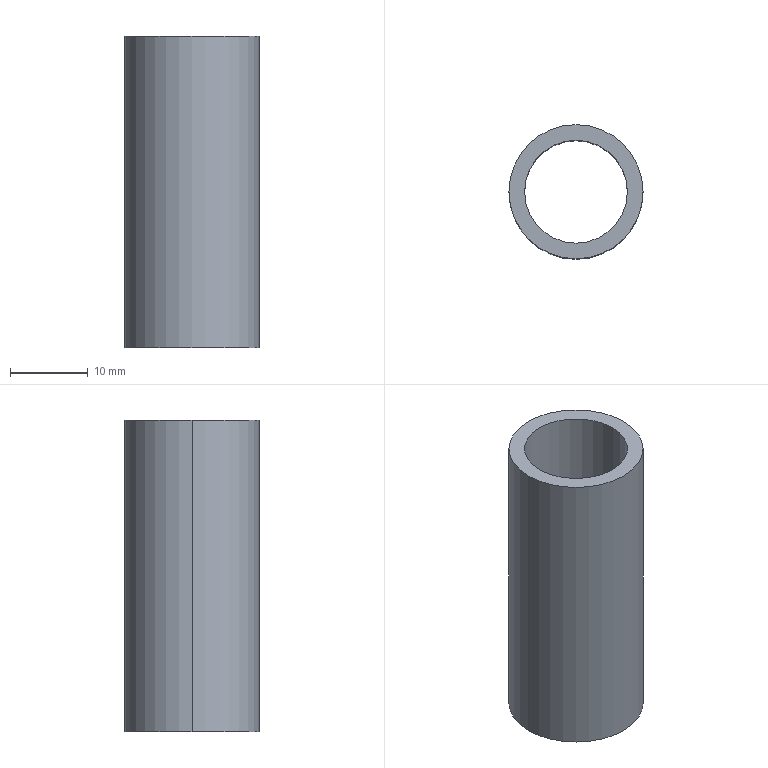Part | STEP file | IN-01-01-01-09 | 1 solid | 6 faces | box 17.2 x 17.2 x 40 mm | volume 3820 mm3 | cylinder 4 | plane 2 | commonest cylinder face diameters 13.2 x2 17.2 x2
STEP:
#1=CARTESIAN_POINT('',(0.,0.,0.));
#2=DIRECTION('',(0.,0.,1.));
#3=DIRECTION('',(1.,0.,0.));
#4=AXIS2_PLACEMENT_3D('',#1,#2,#3);
#5=CARTESIAN_POINT('',(8.6,0.,0.));
#6=VERTEX_POINT('',#5);
#7=CARTESIAN_POINT('',(-8.6,0.,0.));
#8=VERTEX_POINT('',#7);
#9=CARTESIAN_POINT('',(0.,0.,0.));
#10=DIRECTION('',(0.,0.,1.));
#11=DIRECTION('',(1.,0.,0.));
#12=AXIS2_PLACEMENT_3D('',#9,#10,#11);
#13=CIRCLE('',#12,8.6);
#14=CARTESIAN_POINT('',(0.,0.,0.));
#15=DIRECTION('',(0.,0.,1.));
#16=DIRECTION('',(1.,0.,0.));
#17=AXIS2_PLACEMENT_3D('',#14,#15,#16);
#18=CYLINDRICAL_SURFACE('',#17,8.6);
#19=CARTESIAN_POINT('',(0.,0.));
#20=DIRECTION('',(1.,0.));
#21=VECTOR('',#20,1.);
#22=LINE('',#19,#21);
#23=(GEOMETRIC_REPRESENTATION_CONTEXT(2)PARAMETRIC_REPRESENTATION_CONTEXT()REPRESENTATION_CONTEXT('',''));
#24=DEFINITIONAL_REPRESENTATION('',(#22),#23);
#25=PCURVE('',#18,#24);
#26=CARTESIAN_POINT('',(0.,0.,0.));
#27=DIRECTION('',(0.,0.,1.));
#28=DIRECTION('',(1.,0.,0.));
#29=AXIS2_PLACEMENT_3D('',#26,#27,#28);
#30=PLANE('',#29);
#31=CARTESIAN_POINT('',(0.,0.));
#32=DIRECTION('',(1.,0.));
#33=AXIS2_PLACEMENT_2D('',#31,#32);
#34=CIRCLE('',#33,8.6);
#35=(GEOMETRIC_REPRESENTATION_CONTEXT(2)PARAMETRIC_REPRESENTATION_CONTEXT()REPRESENTATION_CONTEXT('',''));
#36=DEFINITIONAL_REPRESENTATION('',(#34),#35);
#37=PCURVE('',#30,#36);
#38=SURFACE_CURVE('',#13,(#25,#37),.PCURVE_S1.);
#39=EDGE_CURVE('',#6,#8,#38,.T.);
#40=ORIENTED_EDGE('',*,*,#39,.T.);
#41=CARTESIAN_POINT('',(-8.6,0.,40.));
#42=VERTEX_POINT('',#41);
#43=CARTESIAN_POINT('',(-8.6,0.,0.));
#44=DIRECTION('',(0.,0.,1.));
#45=VECTOR('',#44,1.);
#46=LINE('',#43,#45);
#47=CARTESIAN_POINT('',(3.142,0.));
#48=DIRECTION('',(0.,1.));
#49=VECTOR('',#48,1.);
#50=LINE('',#47,#49);
#51=(GEOMETRIC_REPRESENTATION_CONTEXT(2)PARAMETRIC_REPRESENTATION_CONTEXT()REPRESENTATION_CONTEXT('',''));
#52=DEFINITIONAL_REPRESENTATION('',(#50),#51);
#53=PCURVE('',#18,#52);
#54=CARTESIAN_POINT('',(0.,0.,0.));
#55=DIRECTION('',(0.,0.,1.));
#56=DIRECTION('',(1.,0.,0.));
#57=AXIS2_PLACEMENT_3D('',#54,#55,#56);
#58=CYLINDRICAL_SURFACE('',#57,8.6);
#59=CARTESIAN_POINT('',(3.142,0.));
#60=DIRECTION('',(0.,1.));
#61=VECTOR('',#60,1.);
#62=LINE('',#59,#61);
#63=(GEOMETRIC_REPRESENTATION_CONTEXT(2)PARAMETRIC_REPRESENTATION_CONTEXT()REPRESENTATION_CONTEXT('',''));
#64=DEFINITIONAL_REPRESENTATION('',(#62),#63);
#65=PCURVE('',#58,#64);
#66=SURFACE_CURVE('',#46,(#53,#65),.PCURVE_S1.);
#67=EDGE_CURVE('',#8,#42,#66,.T.);
#68=ORIENTED_EDGE('',*,*,#67,.T.);
#69=CARTESIAN_POINT('',(8.6,0.,40.));
#70=VERTEX_POINT('',#69);
#71=CARTESIAN_POINT('',(0.,0.,40.));
#72=DIRECTION('',(0.,0.,-1.));
#73=DIRECTION('',(1.,0.,0.));
#74=AXIS2_PLACEMENT_3D('',#71,#72,#73);
#75=CIRCLE('',#74,8.6);
#76=CARTESIAN_POINT('',(6.283,40.));
#77=DIRECTION('',(-1.,0.));
#78=VECTOR('',#77,1.);
#79=LINE('',#76,#78);
#80=(GEOMETRIC_REPRESENTATION_CONTEXT(2)PARAMETRIC_REPRESENTATION_CONTEXT()REPRESENTATION_CONTEXT('',''));
#81=DEFINITIONAL_REPRESENTATION('',(#79),#80);
#82=PCURVE('',#18,#81);
#83=CARTESIAN_POINT('',(0.,0.,40.));
#84=DIRECTION('',(0.,0.,1.));
#85=DIRECTION('',(1.,0.,0.));
#86=AXIS2_PLACEMENT_3D('',#83,#84,#85);
#87=PLANE('',#86);
#88=CARTESIAN_POINT('',(8.6,0.));
#89=CARTESIAN_POINT('',(8.6,-14.896));
#90=CARTESIAN_POINT('',(-4.3,-7.448));
#91=CARTESIAN_POINT('',(-17.2,0.));
#92=CARTESIAN_POINT('',(-4.3,7.448));
#93=CARTESIAN_POINT('',(8.6,14.896));
#94=CARTESIAN_POINT('',(8.6,0.));
#95=(BOUNDED_CURVE()B_SPLINE_CURVE(2,(#88,#89,#90,#91,#92,#93,#94),.UNSPECIFIED.,.T.,.F.)B_SPLINE_CURVE_WITH_KNOTS((1,2,2,2,2,1),(-2.094,0.,2.094,4.189,6.283,8.378),.UNSPECIFIED.)CURVE()GEOMETRIC_REPRESENTATION_ITEM()RATIONAL_B_SPLINE_CURVE((1.,0.5,1.,0.5,1.,0.5,1.))REPRESENTATION_ITEM(''));
#96=(GEOMETRIC_REPRESENTATION_CONTEXT(2)PARAMETRIC_REPRESENTATION_CONTEXT()REPRESENTATION_CONTEXT('',''));
#97=DEFINITIONAL_REPRESENTATION('',(#95),#96);
#98=PCURVE('',#87,#97);
#99=SURFACE_CURVE('',#75,(#82,#98),.PCURVE_S1.);
#100=EDGE_CURVE('',#42,#70,#99,.T.);
#101=ORIENTED_EDGE('',*,*,#100,.T.);
#102=CARTESIAN_POINT('',(8.6,0.,0.));
#103=DIRECTION('',(0.,0.,1.));
#104=VECTOR('',#103,1.);
#105=LINE('',#102,#104);
#106=CARTESIAN_POINT('',(0.,0.));
#107=DIRECTION('',(0.,1.));
#108=VECTOR('',#107,1.);
#109=LINE('',#106,#108);
#110=(GEOMETRIC_REPRESENTATION_CONTEXT(2)PARAMETRIC_REPRESENTATION_CONTEXT()REPRESENTATION_CONTEXT('',''));
#111=DEFINITIONAL_REPRESENTATION('',(#109),#110);
#112=PCURVE('',#18,#111);
#113=CARTESIAN_POINT('',(6.283,0.));
#114=DIRECTION('',(0.,1.));
#115=VECTOR('',#114,1.);
#116=LINE('',#113,#115);
#117=(GEOMETRIC_REPRESENTATION_CONTEXT(2)PARAMETRIC_REPRESENTATION_CONTEXT()REPRESENTATION_CONTEXT('',''));
#118=DEFINITIONAL_REPRESENTATION('',(#116),#117);
#119=PCURVE('',#58,#118);
#120=SURFACE_CURVE('',#105,(#112,#119),.PCURVE_S1.);
#121=EDGE_CURVE('',#6,#70,#120,.T.);
#122=ORIENTED_EDGE('',*,*,#121,.F.);
#123=EDGE_LOOP('',(#40,#68,#101,#122));
#124=FACE_BOUND('',#123,.T.);
#125=ADVANCED_FACE('',(#124),#18,.T.);
#126=CARTESIAN_POINT('',(6.6,0.,0.));
#127=VERTEX_POINT('',#126);
#128=CARTESIAN_POINT('',(6.6,0.,40.));
#129=VERTEX_POINT('',#128);
#130=CARTESIAN_POINT('',(6.6,0.,0.));
#131=DIRECTION('',(0.,0.,1.));
#132=VECTOR('',#131,1.);
#133=LINE('',#130,#132);
#134=CARTESIAN_POINT('',(0.,0.,0.));
#135=DIRECTION('',(0.,0.,1.));
#136=DIRECTION('',(1.,0.,0.));
#137=AXIS2_PLACEMENT_3D('',#134,#135,#136);
#138=CYLINDRICAL_SURFACE('',#137,6.6);
#139=CARTESIAN_POINT('',(6.283,0.));
#140=DIRECTION('',(0.,1.));
#141=VECTOR('',#140,1.);
#142=LINE('',#139,#141);
#143=(GEOMETRIC_REPRESENTATION_CONTEXT(2)PARAMETRIC_REPRESENTATION_CONTEXT()REPRESENTATION_CONTEXT('',''));
#144=DEFINITIONAL_REPRESENTATION('',(#142),#143);
#145=PCURVE('',#138,#144);
#146=CARTESIAN_POINT('',(0.,0.,0.));
#147=DIRECTION('',(0.,0.,1.));
#148=DIRECTION('',(1.,0.,0.));
#149=AXIS2_PLACEMENT_3D('',#146,#147,#148);
#150=CYLINDRICAL_SURFACE('',#149,6.6);
#151=CARTESIAN_POINT('',(0.,0.));
#152=DIRECTION('',(0.,1.));
#153=VECTOR('',#152,1.);
#154=LINE('',#151,#153);
#155=(GEOMETRIC_REPRESENTATION_CONTEXT(2)PARAMETRIC_REPRESENTATION_CONTEXT()REPRESENTATION_CONTEXT('',''));
#156=DEFINITIONAL_REPRESENTATION('',(#154),#155);
#157=PCURVE('',#150,#156);
#158=SURFACE_CURVE('',#133,(#145,#157),.PCURVE_S1.);
#159=EDGE_CURVE('',#127,#129,#158,.T.);
#160=ORIENTED_EDGE('',*,*,#159,.T.);
#161=CARTESIAN_POINT('',(-6.6,0.,40.));
#162=VERTEX_POINT('',#161);
#163=CARTESIAN_POINT('',(0.,0.,40.));
#164=DIRECTION('',(0.,0.,-1.));
#165=DIRECTION('',(1.,0.,0.));
#166=AXIS2_PLACEMENT_3D('',#163,#164,#165);
#167=CIRCLE('',#166,6.6);
#168=CARTESIAN_POINT('',(6.283,40.));
#169=DIRECTION('',(-1.,0.));
#170=VECTOR('',#169,1.);
#171=LINE('',#168,#170);
#172=(GEOMETRIC_REPRESENTATION_CONTEXT(2)PARAMETRIC_REPRESENTATION_CONTEXT()REPRESENTATION_CONTEXT('',''));
#173=DEFINITIONAL_REPRESENTATION('',(#171),#172);
#174=PCURVE('',#138,#173);
#175=CARTESIAN_POINT('',(6.6,0.));
#176=CARTESIAN_POINT('',(6.6,-11.432));
#177=CARTESIAN_POINT('',(-3.3,-5.716));
#178=CARTESIAN_POINT('',(-13.2,0.));
#179=CARTESIAN_POINT('',(-3.3,5.716));
#180=CARTESIAN_POINT('',(6.6,11.432));
#181=CARTESIAN_POINT('',(6.6,0.));
#182=(BOUNDED_CURVE()B_SPLINE_CURVE(2,(#175,#176,#177,#178,#179,#180,#181),.UNSPECIFIED.,.T.,.F.)B_SPLINE_CURVE_WITH_KNOTS((1,2,2,2,2,1),(-2.094,0.,2.094,4.189,6.283,8.378),.UNSPECIFIED.)CURVE()GEOMETRIC_REPRESENTATION_ITEM()RATIONAL_B_SPLINE_CURVE((1.,0.5,1.,0.5,1.,0.5,1.))REPRESENTATION_ITEM(''));
#183=(GEOMETRIC_REPRESENTATION_CONTEXT(2)PARAMETRIC_REPRESENTATION_CONTEXT()REPRESENTATION_CONTEXT('',''));
#184=DEFINITIONAL_REPRESENTATION('',(#182),#183);
#185=PCURVE('',#87,#184);
#186=SURFACE_CURVE('',#167,(#174,#185),.PCURVE_S1.);
#187=EDGE_CURVE('',#129,#162,#186,.T.);
#188=ORIENTED_EDGE('',*,*,#187,.T.);
#189=CARTESIAN_POINT('',(-6.6,0.,0.));
#190=VERTEX_POINT('',#189);
#191=CARTESIAN_POINT('',(-6.6,0.,0.));
#192=DIRECTION('',(0.,0.,1.));
#193=VECTOR('',#192,1.);
#194=LINE('',#191,#193);
#195=CARTESIAN_POINT('',(3.142,0.));
#196=DIRECTION('',(0.,1.));
#197=VECTOR('',#196,1.);
#198=LINE('',#195,#197);
#199=(GEOMETRIC_REPRESENTATION_CONTEXT(2)PARAMETRIC_REPRESENTATION_CONTEXT()REPRESENTATION_CONTEXT('',''));
#200=DEFINITIONAL_REPRESENTATION('',(#198),#199);
#201=PCURVE('',#138,#200);
#202=CARTESIAN_POINT('',(3.142,0.));
#203=DIRECTION('',(0.,1.));
#204=VECTOR('',#203,1.);
#205=LINE('',#202,#204);
#206=(GEOMETRIC_REPRESENTATION_CONTEXT(2)PARAMETRIC_REPRESENTATION_CONTEXT()REPRESENTATION_CONTEXT('',''));
#207=DEFINITIONAL_REPRESENTATION('',(#205),#206);
#208=PCURVE('',#150,#207);
#209=SURFACE_CURVE('',#194,(#201,#208),.PCURVE_S1.);
#210=EDGE_CURVE('',#190,#162,#209,.T.);
#211=ORIENTED_EDGE('',*,*,#210,.F.);
#212=CARTESIAN_POINT('',(0.,0.,0.));
#213=DIRECTION('',(0.,0.,-1.));
#214=DIRECTION('',(1.,0.,0.));
#215=AXIS2_PLACEMENT_3D('',#212,#213,#214);
#216=CIRCLE('',#215,6.6);
#217=CARTESIAN_POINT('',(6.283,0.));
#218=DIRECTION('',(-1.,0.));
#219=VECTOR('',#218,1.);
#220=LINE('',#217,#219);
#221=(GEOMETRIC_REPRESENTATION_CONTEXT(2)PARAMETRIC_REPRESENTATION_CONTEXT()REPRESENTATION_CONTEXT('',''));
#222=DEFINITIONAL_REPRESENTATION('',(#220),#221);
#223=PCURVE('',#138,#222);
#224=CARTESIAN_POINT('',(6.6,0.));
#225=CARTESIAN_POINT('',(6.6,-11.432));
#226=CARTESIAN_POINT('',(-3.3,-5.716));
#227=CARTESIAN_POINT('',(-13.2,0.));
#228=CARTESIAN_POINT('',(-3.3,5.716));
#229=CARTESIAN_POINT('',(6.6,11.432));
#230=CARTESIAN_POINT('',(6.6,0.));
#231=(BOUNDED_CURVE()B_SPLINE_CURVE(2,(#224,#225,#226,#227,#228,#229,#230),.UNSPECIFIED.,.T.,.F.)B_SPLINE_CURVE_WITH_KNOTS((1,2,2,2,2,1),(-2.094,0.,2.094,4.189,6.283,8.378),.UNSPECIFIED.)CURVE()GEOMETRIC_REPRESENTATION_ITEM()RATIONAL_B_SPLINE_CURVE((1.,0.5,1.,0.5,1.,0.5,1.))REPRESENTATION_ITEM(''));
#232=(GEOMETRIC_REPRESENTATION_CONTEXT(2)PARAMETRIC_REPRESENTATION_CONTEXT()REPRESENTATION_CONTEXT('',''));
#233=DEFINITIONAL_REPRESENTATION('',(#231),#232);
#234=PCURVE('',#30,#233);
#235=SURFACE_CURVE('',#216,(#223,#234),.PCURVE_S1.);
#236=EDGE_CURVE('',#127,#190,#235,.T.);
#237=ORIENTED_EDGE('',*,*,#236,.F.);
#238=EDGE_LOOP('',(#160,#188,#211,#237));
#239=FACE_BOUND('',#238,.F.);
#240=ADVANCED_FACE('',(#239),#138,.F.);
#241=ORIENTED_EDGE('',*,*,#67,.F.);
#242=CARTESIAN_POINT('',(0.,0.,0.));
#243=DIRECTION('',(0.,0.,1.));
#244=DIRECTION('',(1.,0.,0.));
#245=AXIS2_PLACEMENT_3D('',#242,#243,#244);
#246=CIRCLE('',#245,8.6);
#247=CARTESIAN_POINT('',(0.,0.));
#248=DIRECTION('',(1.,0.));
#249=VECTOR('',#248,1.);
#250=LINE('',#247,#249);
#251=(GEOMETRIC_REPRESENTATION_CONTEXT(2)PARAMETRIC_REPRESENTATION_CONTEXT()REPRESENTATION_CONTEXT('',''));
#252=DEFINITIONAL_REPRESENTATION('',(#250),#251);
#253=PCURVE('',#58,#252);
#254=CARTESIAN_POINT('',(0.,0.));
#255=DIRECTION('',(1.,0.));
#256=AXIS2_PLACEMENT_2D('',#254,#255);
#257=CIRCLE('',#256,8.6);
#258=(GEOMETRIC_REPRESENTATION_CONTEXT(2)PARAMETRIC_REPRESENTATION_CONTEXT()REPRESENTATION_CONTEXT('',''));
#259=DEFINITIONAL_REPRESENTATION('',(#257),#258);
#260=PCURVE('',#30,#259);
#261=SURFACE_CURVE('',#246,(#253,#260),.PCURVE_S1.);
#262=EDGE_CURVE('',#8,#6,#261,.T.);
#263=ORIENTED_EDGE('',*,*,#262,.T.);
#264=ORIENTED_EDGE('',*,*,#121,.T.);
#265=CARTESIAN_POINT('',(0.,0.,40.));
#266=DIRECTION('',(0.,0.,-1.));
#267=DIRECTION('',(1.,0.,0.));
#268=AXIS2_PLACEMENT_3D('',#265,#266,#267);
#269=CIRCLE('',#268,8.6);
#270=CARTESIAN_POINT('',(6.283,40.));
#271=DIRECTION('',(-1.,0.));
#272=VECTOR('',#271,1.);
#273=LINE('',#270,#272);
#274=(GEOMETRIC_REPRESENTATION_CONTEXT(2)PARAMETRIC_REPRESENTATION_CONTEXT()REPRESENTATION_CONTEXT('',''));
#275=DEFINITIONAL_REPRESENTATION('',(#273),#274);
#276=PCURVE('',#58,#275);
#277=CARTESIAN_POINT('',(8.6,0.));
#278=CARTESIAN_POINT('',(8.6,-14.896));
#279=CARTESIAN_POINT('',(-4.3,-7.448));
#280=CARTESIAN_POINT('',(-17.2,0.));
#281=CARTESIAN_POINT('',(-4.3,7.448));
#282=CARTESIAN_POINT('',(8.6,14.896));
#283=CARTESIAN_POINT('',(8.6,0.));
#284=(BOUNDED_CURVE()B_SPLINE_CURVE(2,(#277,#278,#279,#280,#281,#282,#283),.UNSPECIFIED.,.T.,.F.)B_SPLINE_CURVE_WITH_KNOTS((1,2,2,2,2,1),(-2.094,0.,2.094,4.189,6.283,8.378),.UNSPECIFIED.)CURVE()GEOMETRIC_REPRESENTATION_ITEM()RATIONAL_B_SPLINE_CURVE((1.,0.5,1.,0.5,1.,0.5,1.))REPRESENTATION_ITEM(''));
#285=(GEOMETRIC_REPRESENTATION_CONTEXT(2)PARAMETRIC_REPRESENTATION_CONTEXT()REPRESENTATION_CONTEXT('',''));
#286=DEFINITIONAL_REPRESENTATION('',(#284),#285);
#287=PCURVE('',#87,#286);
#288=SURFACE_CURVE('',#269,(#276,#287),.PCURVE_S1.);
#289=EDGE_CURVE('',#70,#42,#288,.T.);
#290=ORIENTED_EDGE('',*,*,#289,.T.);
#291=EDGE_LOOP('',(#241,#263,#264,#290));
#292=FACE_BOUND('',#291,.T.);
#293=ADVANCED_FACE('',(#292),#58,.T.);
#294=ORIENTED_EDGE('',*,*,#236,.F.);
#295=CARTESIAN_POINT('',(0.,0.,0.));
#296=DIRECTION('',(0.,0.,-1.));
#297=DIRECTION('',(1.,0.,0.));
#298=AXIS2_PLACEMENT_3D('',#295,#296,#297);
#299=CIRCLE('',#298,6.6);
#300=CARTESIAN_POINT('',(6.6,0.));
#301=CARTESIAN_POINT('',(6.6,-11.432));
#302=CARTESIAN_POINT('',(-3.3,-5.716));
#303=CARTESIAN_POINT('',(-13.2,0.));
#304=CARTESIAN_POINT('',(-3.3,5.716));
#305=CARTESIAN_POINT('',(6.6,11.432));
#306=CARTESIAN_POINT('',(6.6,0.));
#307=(BOUNDED_CURVE()B_SPLINE_CURVE(2,(#300,#301,#302,#303,#304,#305,#306),.UNSPECIFIED.,.T.,.F.)B_SPLINE_CURVE_WITH_KNOTS((1,2,2,2,2,1),(-2.094,0.,2.094,4.189,6.283,8.378),.UNSPECIFIED.)CURVE()GEOMETRIC_REPRESENTATION_ITEM()RATIONAL_B_SPLINE_CURVE((1.,0.5,1.,0.5,1.,0.5,1.))REPRESENTATION_ITEM(''));
#308=(GEOMETRIC_REPRESENTATION_CONTEXT(2)PARAMETRIC_REPRESENTATION_CONTEXT()REPRESENTATION_CONTEXT('',''));
#309=DEFINITIONAL_REPRESENTATION('',(#307),#308);
#310=PCURVE('',#30,#309);
#311=CARTESIAN_POINT('',(6.283,0.));
#312=DIRECTION('',(-1.,0.));
#313=VECTOR('',#312,1.);
#314=LINE('',#311,#313);
#315=(GEOMETRIC_REPRESENTATION_CONTEXT(2)PARAMETRIC_REPRESENTATION_CONTEXT()REPRESENTATION_CONTEXT('',''));
#316=DEFINITIONAL_REPRESENTATION('',(#314),#315);
#317=PCURVE('',#150,#316);
#318=SURFACE_CURVE('',#299,(#310,#317),.PCURVE_S1.);
#319=EDGE_CURVE('',#190,#127,#318,.T.);
#320=ORIENTED_EDGE('',*,*,#319,.F.);
#321=EDGE_LOOP('',(#294,#320));
#322=FACE_BOUND('',#321,.T.);
#323=ORIENTED_EDGE('',*,*,#39,.F.);
#324=ORIENTED_EDGE('',*,*,#262,.F.);
#325=EDGE_LOOP('',(#323,#324));
#326=FACE_BOUND('',#325,.T.);
#327=ADVANCED_FACE('',(#322,#326),#30,.F.);
#328=ORIENTED_EDGE('',*,*,#187,.T.);
#329=CARTESIAN_POINT('',(0.,0.,40.));
#330=DIRECTION('',(0.,0.,-1.));
#331=DIRECTION('',(1.,0.,0.));
#332=AXIS2_PLACEMENT_3D('',#329,#330,#331);
#333=CIRCLE('',#332,6.6);
#334=CARTESIAN_POINT('',(6.6,0.));
#335=CARTESIAN_POINT('',(6.6,-11.432));
#336=CARTESIAN_POINT('',(-3.3,-5.716));
#337=CARTESIAN_POINT('',(-13.2,0.));
#338=CARTESIAN_POINT('',(-3.3,5.716));
#339=CARTESIAN_POINT('',(6.6,11.432));
#340=CARTESIAN_POINT('',(6.6,0.));
#341=(BOUNDED_CURVE()B_SPLINE_CURVE(2,(#334,#335,#336,#337,#338,#339,#340),.UNSPECIFIED.,.T.,.F.)B_SPLINE_CURVE_WITH_KNOTS((1,2,2,2,2,1),(-2.094,0.,2.094,4.189,6.283,8.378),.UNSPECIFIED.)CURVE()GEOMETRIC_REPRESENTATION_ITEM()RATIONAL_B_SPLINE_CURVE((1.,0.5,1.,0.5,1.,0.5,1.))REPRESENTATION_ITEM(''));
#342=(GEOMETRIC_REPRESENTATION_CONTEXT(2)PARAMETRIC_REPRESENTATION_CONTEXT()REPRESENTATION_CONTEXT('',''));
#343=DEFINITIONAL_REPRESENTATION('',(#341),#342);
#344=PCURVE('',#87,#343);
#345=CARTESIAN_POINT('',(6.283,40.));
#346=DIRECTION('',(-1.,0.));
#347=VECTOR('',#346,1.);
#348=LINE('',#345,#347);
#349=(GEOMETRIC_REPRESENTATION_CONTEXT(2)PARAMETRIC_REPRESENTATION_CONTEXT()REPRESENTATION_CONTEXT('',''));
#350=DEFINITIONAL_REPRESENTATION('',(#348),#349);
#351=PCURVE('',#150,#350);
#352=SURFACE_CURVE('',#333,(#344,#351),.PCURVE_S1.);
#353=EDGE_CURVE('',#162,#129,#352,.T.);
#354=ORIENTED_EDGE('',*,*,#353,.T.);
#355=EDGE_LOOP('',(#328,#354));
#356=FACE_BOUND('',#355,.T.);
#357=ORIENTED_EDGE('',*,*,#289,.F.);
#358=ORIENTED_EDGE('',*,*,#100,.F.);
#359=EDGE_LOOP('',(#357,#358));
#360=FACE_BOUND('',#359,.T.);
#361=ADVANCED_FACE('',(#356,#360),#87,.T.);
#362=ORIENTED_EDGE('',*,*,#353,.T.);
#363=ORIENTED_EDGE('',*,*,#159,.F.);
#364=ORIENTED_EDGE('',*,*,#319,.F.);
#365=ORIENTED_EDGE('',*,*,#210,.T.);
#366=EDGE_LOOP('',(#362,#363,#364,#365));
#367=FACE_BOUND('',#366,.F.);
#368=ADVANCED_FACE('',(#367),#150,.F.);
#369=CLOSED_SHELL('',(#125,#240,#293,#327,#361,#368));
#370=MANIFOLD_SOLID_BREP('',#369);
#371=(LENGTH_UNIT()NAMED_UNIT(*)SI_UNIT(.MILLI.,.METRE.));
#372=UNCERTAINTY_MEASURE_WITH_UNIT(LENGTH_MEASURE(0.0000001),#371,'','');
#373=(NAMED_UNIT(*)PLANE_ANGLE_UNIT()SI_UNIT($,.RADIAN.));
#374=(NAMED_UNIT(*)SI_UNIT($,.STERADIAN.)SOLID_ANGLE_UNIT());
#375=(GEOMETRIC_REPRESENTATION_CONTEXT(3)GLOBAL_UNCERTAINTY_ASSIGNED_CONTEXT((#372))GLOBAL_UNIT_ASSIGNED_CONTEXT((#371,#373,#374))REPRESENTATION_CONTEXT('',''));
#376=ADVANCED_BREP_SHAPE_REPRESENTATION('',(#4,#370),#375);